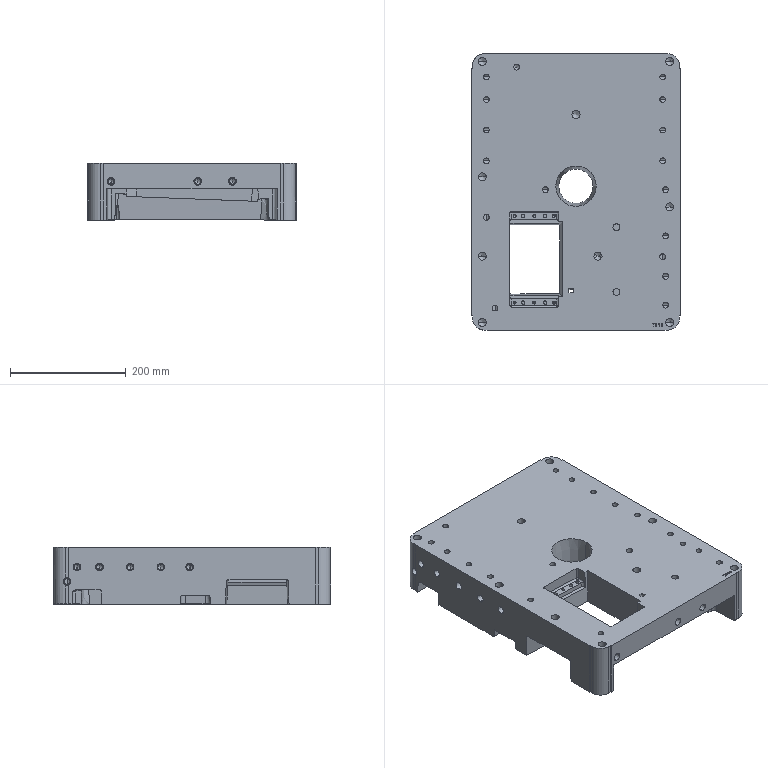Part | Creo | 1 solid | 657 faces | box 360 x 480.001 x 99.001 mm | volume 10654704 mm3 | plane 254 | cylinder 188 | cone 132 | other 64 | spline 12 | sphere 6 | torus 1 | commonest cylinder face diameters 10 x82 6 x22 8 x20 14 x18 5.1 x12 1.004 x6